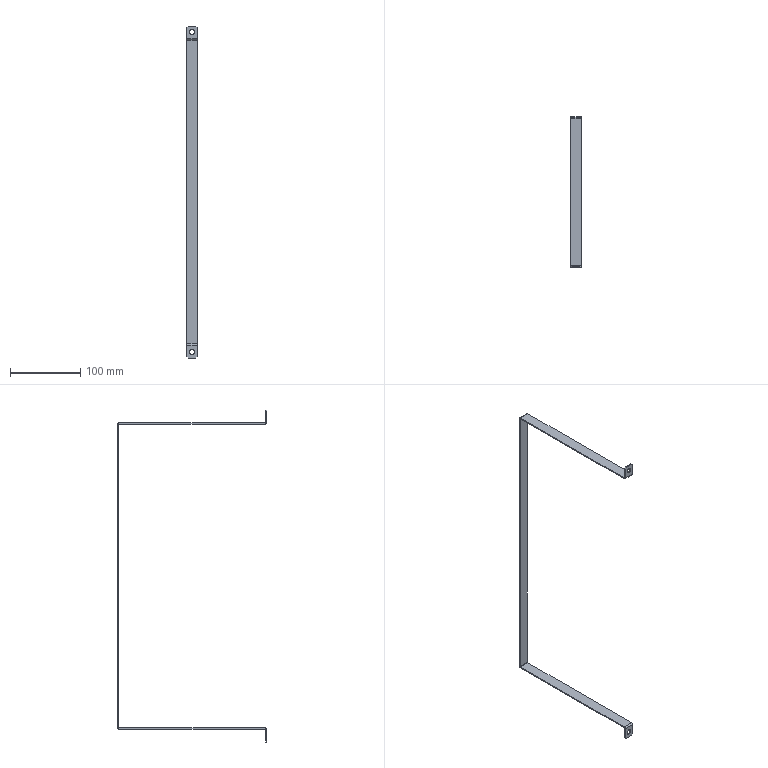Part | SolidWorks | features BaseBody 1 | 1 solid | 30 faces | box 15 x 213.5 x 473 mm | volume 19998 mm3 | plane 18 | cylinder 12 | commonest cylinder face diameters 1.473 x4 4.473 x4 7 x4
STEP:
#1=CARTESIAN_POINT('',(0.,1.5,-231.5));
#2=VERTEX_POINT('',#1);
#3=CARTESIAN_POINT('',(0.,1.5,-224.5));
#4=VERTEX_POINT('',#3);
#5=CARTESIAN_POINT('',(0.,1.5,-228.));
#6=DIRECTION('',(0.,1.,0.));
#7=DIRECTION('',(0.,0.,-1.));
#8=AXIS2_PLACEMENT_3D('',#5,#6,#7);
#9=CIRCLE('',#8,3.5);
#10=EDGE_CURVE('',#2,#4,#9,.T.);
#11=ORIENTED_EDGE('',*,*,#10,.T.);
#12=CARTESIAN_POINT('',(0.,0.,-224.5));
#13=VERTEX_POINT('',#12);
#14=CARTESIAN_POINT('',(0.,213.501,-224.5));
#15=DIRECTION('',(0.,-1.,0.));
#16=VECTOR('',#15,1000.);
#17=LINE('',#14,#16);
#18=EDGE_CURVE('',#4,#13,#17,.T.);
#19=ORIENTED_EDGE('',*,*,#18,.T.);
#20=CARTESIAN_POINT('',(0.,0.,-231.5));
#21=VERTEX_POINT('',#20);
#22=CARTESIAN_POINT('',(0.,0.,-228.));
#23=DIRECTION('',(0.,-1.,0.));
#24=DIRECTION('',(0.,0.,1.));
#25=AXIS2_PLACEMENT_3D('',#22,#23,#24);
#26=CIRCLE('',#25,3.5);
#27=EDGE_CURVE('',#13,#21,#26,.T.);
#28=ORIENTED_EDGE('',*,*,#27,.T.);
#29=CARTESIAN_POINT('',(0.,213.501,-231.5));
#30=DIRECTION('',(0.,-1.,0.));
#31=VECTOR('',#30,1000.);
#32=LINE('',#29,#31);
#33=EDGE_CURVE('',#2,#21,#32,.T.);
#34=ORIENTED_EDGE('',*,*,#33,.F.);
#35=EDGE_LOOP('',(#11,#19,#28,#34));
#36=FACE_OUTER_BOUND('',#35,.T.);
#37=CARTESIAN_POINT('',(0.,213.501,-228.));
#38=DIRECTION('',(0.,-1.,0.));
#39=DIRECTION('',(0.,0.,-1.));
#40=AXIS2_PLACEMENT_3D('',#37,#38,#39);
#41=CYLINDRICAL_SURFACE('',#40,3.5);
#42=ADVANCED_FACE('',(#36),#41,.F.);
#43=CARTESIAN_POINT('',(0.,1.5,224.5));
#44=VERTEX_POINT('',#43);
#45=CARTESIAN_POINT('',(0.,1.5,231.5));
#46=VERTEX_POINT('',#45);
#47=CARTESIAN_POINT('',(0.,1.5,228.));
#48=DIRECTION('',(0.,1.,0.));
#49=DIRECTION('',(0.,0.,-1.));
#50=AXIS2_PLACEMENT_3D('',#47,#48,#49);
#51=CIRCLE('',#50,3.5);
#52=EDGE_CURVE('',#44,#46,#51,.T.);
#53=ORIENTED_EDGE('',*,*,#52,.T.);
#54=CARTESIAN_POINT('',(0.,0.,231.5));
#55=VERTEX_POINT('',#54);
#56=CARTESIAN_POINT('',(0.,213.501,231.5));
#57=DIRECTION('',(0.,-1.,0.));
#58=VECTOR('',#57,1000.);
#59=LINE('',#56,#58);
#60=EDGE_CURVE('',#46,#55,#59,.T.);
#61=ORIENTED_EDGE('',*,*,#60,.T.);
#62=CARTESIAN_POINT('',(0.,0.,224.5));
#63=VERTEX_POINT('',#62);
#64=CARTESIAN_POINT('',(0.,0.,228.));
#65=DIRECTION('',(0.,-1.,0.));
#66=DIRECTION('',(0.,0.,-1.));
#67=AXIS2_PLACEMENT_3D('',#64,#65,#66);
#68=CIRCLE('',#67,3.5);
#69=EDGE_CURVE('',#55,#63,#68,.T.);
#70=ORIENTED_EDGE('',*,*,#69,.T.);
#71=CARTESIAN_POINT('',(0.,213.501,224.5));
#72=DIRECTION('',(0.,-1.,0.));
#73=VECTOR('',#72,1000.);
#74=LINE('',#71,#73);
#75=EDGE_CURVE('',#44,#63,#74,.T.);
#76=ORIENTED_EDGE('',*,*,#75,.F.);
#77=EDGE_LOOP('',(#53,#61,#70,#76));
#78=FACE_OUTER_BOUND('',#77,.T.);
#79=CARTESIAN_POINT('',(0.,213.501,228.));
#80=DIRECTION('',(0.,-1.,0.));
#81=DIRECTION('',(0.,0.,-1.));
#82=AXIS2_PLACEMENT_3D('',#79,#80,#81);
#83=CYLINDRICAL_SURFACE('',#82,3.5);
#84=ADVANCED_FACE('',(#78),#83,.F.);
#85=CARTESIAN_POINT('',(-5.5,0.,236.5));
#86=VERTEX_POINT('',#85);
#87=CARTESIAN_POINT('',(-7.5,0.,234.5));
#88=VERTEX_POINT('',#87);
#89=CARTESIAN_POINT('',(1.,0.,243.));
#90=DIRECTION('',(-0.7071,0.,-0.7071));
#91=VECTOR('',#90,1000.);
#92=LINE('',#89,#91);
#93=EDGE_CURVE('',#86,#88,#92,.T.);
#94=ORIENTED_EDGE('',*,*,#93,.F.);
#95=CARTESIAN_POINT('',(-5.5,1.5,236.5));
#96=VERTEX_POINT('',#95);
#97=CARTESIAN_POINT('',(-5.5,0.,236.5));
#98=DIRECTION('',(0.,-1.,0.));
#99=VECTOR('',#98,1000.);
#100=LINE('',#97,#99);
#101=EDGE_CURVE('',#96,#86,#100,.T.);
#102=ORIENTED_EDGE('',*,*,#101,.F.);
#103=CARTESIAN_POINT('',(-7.5,1.5,234.5));
#104=VERTEX_POINT('',#103);
#105=CARTESIAN_POINT('',(-7.5,1.5,234.5));
#106=DIRECTION('',(0.7071,0.,0.7071));
#107=VECTOR('',#106,1000.);
#108=LINE('',#105,#107);
#109=EDGE_CURVE('',#104,#96,#108,.T.);
#110=ORIENTED_EDGE('',*,*,#109,.F.);
#111=CARTESIAN_POINT('',(-7.5,2.237,234.5));
#112=DIRECTION('',(0.,1.,0.));
#113=VECTOR('',#112,1000.);
#114=LINE('',#111,#113);
#115=EDGE_CURVE('',#88,#104,#114,.T.);
#116=ORIENTED_EDGE('',*,*,#115,.F.);
#117=EDGE_LOOP('',(#94,#102,#110,#116));
#118=FACE_OUTER_BOUND('',#117,.T.);
#119=CARTESIAN_POINT('',(-7.5,2.237,234.5));
#120=DIRECTION('',(0.7071,0.,-0.7071));
#121=DIRECTION('',(0.,-1.,0.));
#122=AXIS2_PLACEMENT_3D('',#119,#120,#121);
#123=PLANE('',#122);
#124=ADVANCED_FACE('',(#118),#123,.F.);
#125=CARTESIAN_POINT('',(7.5,0.,234.5));
#126=VERTEX_POINT('',#125);
#127=CARTESIAN_POINT('',(5.5,0.,236.5));
#128=VERTEX_POINT('',#127);
#129=CARTESIAN_POINT('',(6.5,0.,235.5));
#130=DIRECTION('',(-0.7071,0.,0.7071));
#131=VECTOR('',#130,1000.);
#132=LINE('',#129,#131);
#133=EDGE_CURVE('',#126,#128,#132,.T.);
#134=ORIENTED_EDGE('',*,*,#133,.F.);
#135=CARTESIAN_POINT('',(7.5,1.5,234.5));
#136=VERTEX_POINT('',#135);
#137=CARTESIAN_POINT('',(7.5,2.237,234.5));
#138=DIRECTION('',(0.,-1.,0.));
#139=VECTOR('',#138,1000.);
#140=LINE('',#137,#139);
#141=EDGE_CURVE('',#136,#126,#140,.T.);
#142=ORIENTED_EDGE('',*,*,#141,.F.);
#143=CARTESIAN_POINT('',(5.5,1.5,236.5));
#144=VERTEX_POINT('',#143);
#145=CARTESIAN_POINT('',(5.5,1.5,236.5));
#146=DIRECTION('',(0.7071,0.,-0.7071));
#147=VECTOR('',#146,1000.);
#148=LINE('',#145,#147);
#149=EDGE_CURVE('',#144,#136,#148,.T.);
#150=ORIENTED_EDGE('',*,*,#149,.F.);
#151=CARTESIAN_POINT('',(5.5,0.,236.5));
#152=DIRECTION('',(0.,1.,0.));
#153=VECTOR('',#152,1000.);
#154=LINE('',#151,#153);
#155=EDGE_CURVE('',#128,#144,#154,.T.);
#156=ORIENTED_EDGE('',*,*,#155,.F.);
#157=EDGE_LOOP('',(#134,#142,#150,#156));
#158=FACE_OUTER_BOUND('',#157,.T.);
#159=CARTESIAN_POINT('',(5.5,0.,236.5));
#160=DIRECTION('',(-0.7071,0.,-0.7071));
#161=DIRECTION('',(-0.7071,0.,0.7071));
#162=AXIS2_PLACEMENT_3D('',#159,#160,#161);
#163=PLANE('',#162);
#164=ADVANCED_FACE('',(#158),#163,.F.);
#165=CARTESIAN_POINT('',(-5.5,1.5,-236.5));
#166=VERTEX_POINT('',#165);
#167=CARTESIAN_POINT('',(-7.5,1.5,-234.5));
#168=VERTEX_POINT('',#167);
#169=CARTESIAN_POINT('',(-7.5,1.5,-234.5));
#170=DIRECTION('',(-0.7071,0.,0.7071));
#171=VECTOR('',#170,1000.);
#172=LINE('',#169,#171);
#173=EDGE_CURVE('',#166,#168,#172,.T.);
#174=ORIENTED_EDGE('',*,*,#173,.F.);
#175=CARTESIAN_POINT('',(-5.5,0.,-236.5));
#176=VERTEX_POINT('',#175);
#177=CARTESIAN_POINT('',(-5.5,1.5,-236.5));
#178=DIRECTION('',(0.,1.,0.));
#179=VECTOR('',#178,1000.);
#180=LINE('',#177,#179);
#181=EDGE_CURVE('',#176,#166,#180,.T.);
#182=ORIENTED_EDGE('',*,*,#181,.F.);
#183=CARTESIAN_POINT('',(-7.5,0.,-234.5));
#184=VERTEX_POINT('',#183);
#185=CARTESIAN_POINT('',(1.,0.,-243.));
#186=DIRECTION('',(0.7071,0.,-0.7071));
#187=VECTOR('',#186,1000.);
#188=LINE('',#185,#187);
#189=EDGE_CURVE('',#184,#176,#188,.T.);
#190=ORIENTED_EDGE('',*,*,#189,.F.);
#191=CARTESIAN_POINT('',(-7.5,2.237,-234.5));
#192=DIRECTION('',(0.,-1.,0.));
#193=VECTOR('',#192,1000.);
#194=LINE('',#191,#193);
#195=EDGE_CURVE('',#168,#184,#194,.T.);
#196=ORIENTED_EDGE('',*,*,#195,.F.);
#197=EDGE_LOOP('',(#174,#182,#190,#196));
#198=FACE_OUTER_BOUND('',#197,.T.);
#199=CARTESIAN_POINT('',(-7.5,2.237,-234.5));
#200=DIRECTION('',(0.7071,0.,0.7071));
#201=DIRECTION('',(0.,-1.,0.));
#202=AXIS2_PLACEMENT_3D('',#199,#200,#201);
#203=PLANE('',#202);
#204=ADVANCED_FACE('',(#198),#203,.F.);
#205=CARTESIAN_POINT('',(7.5,1.5,-234.5));
#206=VERTEX_POINT('',#205);
#207=CARTESIAN_POINT('',(5.5,1.5,-236.5));
#208=VERTEX_POINT('',#207);
#209=CARTESIAN_POINT('',(5.5,1.5,-236.5));
#210=DIRECTION('',(-0.7071,0.,-0.7071));
#211=VECTOR('',#210,1000.);
#212=LINE('',#209,#211);
#213=EDGE_CURVE('',#206,#208,#212,.T.);
#214=ORIENTED_EDGE('',*,*,#213,.F.);
#215=CARTESIAN_POINT('',(7.5,0.,-234.5));
#216=VERTEX_POINT('',#215);
#217=CARTESIAN_POINT('',(7.5,1.5,-234.5));
#218=DIRECTION('',(0.,1.,0.));
#219=VECTOR('',#218,1000.);
#220=LINE('',#217,#219);
#221=EDGE_CURVE('',#216,#206,#220,.T.);
#222=ORIENTED_EDGE('',*,*,#221,.F.);
#223=CARTESIAN_POINT('',(5.5,0.,-236.5));
#224=VERTEX_POINT('',#223);
#225=CARTESIAN_POINT('',(6.5,0.,-235.5));
#226=DIRECTION('',(0.7071,0.,0.7071));
#227=VECTOR('',#226,1000.);
#228=LINE('',#225,#227);
#229=EDGE_CURVE('',#224,#216,#228,.T.);
#230=ORIENTED_EDGE('',*,*,#229,.F.);
#231=CARTESIAN_POINT('',(5.5,0.,-236.5));
#232=DIRECTION('',(0.,-1.,0.));
#233=VECTOR('',#232,1000.);
#234=LINE('',#231,#233);
#235=EDGE_CURVE('',#208,#224,#234,.T.);
#236=ORIENTED_EDGE('',*,*,#235,.F.);
#237=EDGE_LOOP('',(#214,#222,#230,#236));
#238=FACE_OUTER_BOUND('',#237,.T.);
#239=CARTESIAN_POINT('',(5.5,1.5,-236.5));
#240=DIRECTION('',(0.7071,0.,-0.7071));
#241=DIRECTION('',(0.,-1.,0.));
#242=AXIS2_PLACEMENT_3D('',#239,#240,#241);
#243=PLANE('',#242);
#244=ADVANCED_FACE('',(#238),#243,.T.);
#245=CARTESIAN_POINT('',(-7.5,2.237,218.));
#246=VERTEX_POINT('',#245);
#247=CARTESIAN_POINT('',(-7.5,1.5,218.737));
#248=VERTEX_POINT('',#247);
#249=CARTESIAN_POINT('',(-7.5,2.237,218.737));
#250=DIRECTION('',(-1.,0.,0.));
#251=DIRECTION('',(0.,0.,-1.));
#252=AXIS2_PLACEMENT_3D('',#249,#250,#251);
#253=CIRCLE('',#252,0.7366);
#254=EDGE_CURVE('',#246,#248,#253,.T.);
#255=ORIENTED_EDGE('',*,*,#254,.T.);
#256=CARTESIAN_POINT('',(7.5,1.5,218.737));
#257=VERTEX_POINT('',#256);
#258=CARTESIAN_POINT('',(7.5,1.5,218.737));
#259=DIRECTION('',(-1.,0.,0.));
#260=VECTOR('',#259,1000.);
#261=LINE('',#258,#260);
#262=EDGE_CURVE('',#257,#248,#261,.T.);
#263=ORIENTED_EDGE('',*,*,#262,.F.);
#264=CARTESIAN_POINT('',(7.5,2.237,218.));
#265=VERTEX_POINT('',#264);
#266=CARTESIAN_POINT('',(7.5,2.237,218.737));
#267=DIRECTION('',(-1.,0.,0.));
#268=DIRECTION('',(0.,0.,-1.));
#269=AXIS2_PLACEMENT_3D('',#266,#267,#268);
#270=CIRCLE('',#269,0.7366);
#271=EDGE_CURVE('',#265,#257,#270,.T.);
#272=ORIENTED_EDGE('',*,*,#271,.F.);
#273=CARTESIAN_POINT('',(7.5,2.237,218.));
#274=DIRECTION('',(-1.,0.,0.));
#275=VECTOR('',#274,1000.);
#276=LINE('',#273,#275);
#277=EDGE_CURVE('',#265,#246,#276,.T.);
#278=ORIENTED_EDGE('',*,*,#277,.T.);
#279=EDGE_LOOP('',(#255,#263,#272,#278));
#280=FACE_OUTER_BOUND('',#279,.T.);
#281=CARTESIAN_POINT('',(7.5,2.237,218.737));
#282=DIRECTION('',(-1.,0.,0.));
#283=DIRECTION('',(0.,0.,1.));
#284=AXIS2_PLACEMENT_3D('',#281,#282,#283);
#285=CYLINDRICAL_SURFACE('',#284,0.7366);
#286=ADVANCED_FACE('',(#280),#285,.F.);
#287=CARTESIAN_POINT('',(-7.5,211.263,218.));
#288=VERTEX_POINT('',#287);
#289=CARTESIAN_POINT('',(-7.5,0.,218.));
#290=DIRECTION('',(0.,-1.,0.));
#291=VECTOR('',#290,1000.);
#292=LINE('',#289,#291);
#293=EDGE_CURVE('',#288,#246,#292,.T.);
#294=ORIENTED_EDGE('',*,*,#293,.T.);
#295=ORIENTED_EDGE('',*,*,#277,.F.);
#296=CARTESIAN_POINT('',(7.5,211.263,218.));
#297=VERTEX_POINT('',#296);
#298=CARTESIAN_POINT('',(7.5,0.,218.));
#299=DIRECTION('',(0.,-1.,0.));
#300=VECTOR('',#299,1000.);
#301=LINE('',#298,#300);
#302=EDGE_CURVE('',#297,#265,#301,.T.);
#303=ORIENTED_EDGE('',*,*,#302,.F.);
#304=CARTESIAN_POINT('',(7.5,211.263,218.));
#305=DIRECTION('',(-1.,0.,0.));
#306=VECTOR('',#305,1000.);
#307=LINE('',#304,#306);
#308=EDGE_CURVE('',#297,#288,#307,.T.);
#309=ORIENTED_EDGE('',*,*,#308,.T.);
#310=EDGE_LOOP('',(#294,#295,#303,#309));
#311=FACE_OUTER_BOUND('',#310,.T.);
#312=CARTESIAN_POINT('',(7.5,0.,218.));
#313=DIRECTION('',(0.,0.,-1.));
#314=DIRECTION('',(0.,-1.,0.));
#315=AXIS2_PLACEMENT_3D('',#312,#313,#314);
#316=PLANE('',#315);
#317=ADVANCED_FACE('',(#311),#316,.F.);
#318=CARTESIAN_POINT('',(-7.5,213.5,215.763));
#319=VERTEX_POINT('',#318);
#320=CARTESIAN_POINT('',(-7.5,211.263,215.763));
#321=DIRECTION('',(1.,0.,0.));
#322=DIRECTION('',(0.,0.,-1.));
#323=AXIS2_PLACEMENT_3D('',#320,#321,#322);
#324=CIRCLE('',#323,2.237);
#325=EDGE_CURVE('',#319,#288,#324,.T.);
#326=ORIENTED_EDGE('',*,*,#325,.T.);
#327=ORIENTED_EDGE('',*,*,#308,.F.);
#328=CARTESIAN_POINT('',(7.5,213.5,215.763));
#329=VERTEX_POINT('',#328);
#330=CARTESIAN_POINT('',(7.5,211.263,215.763));
#331=DIRECTION('',(1.,0.,0.));
#332=DIRECTION('',(0.,0.,-1.));
#333=AXIS2_PLACEMENT_3D('',#330,#331,#332);
#334=CIRCLE('',#333,2.237);
#335=EDGE_CURVE('',#329,#297,#334,.T.);
#336=ORIENTED_EDGE('',*,*,#335,.F.);
#337=CARTESIAN_POINT('',(7.5,213.5,215.763));
#338=DIRECTION('',(-1.,0.,0.));
#339=VECTOR('',#338,1000.);
#340=LINE('',#337,#339);
#341=EDGE_CURVE('',#329,#319,#340,.T.);
#342=ORIENTED_EDGE('',*,*,#341,.T.);
#343=EDGE_LOOP('',(#326,#327,#336,#342));
#344=FACE_OUTER_BOUND('',#343,.T.);
#345=CARTESIAN_POINT('',(7.5,211.263,215.763));
#346=DIRECTION('',(-1.,0.,0.));
#347=DIRECTION('',(0.,0.,1.));
#348=AXIS2_PLACEMENT_3D('',#345,#346,#347);
#349=CYLINDRICAL_SURFACE('',#348,2.237);
#350=ADVANCED_FACE('',(#344),#349,.T.);
#351=CARTESIAN_POINT('',(-7.5,213.5,-215.763));
#352=VERTEX_POINT('',#351);
#353=CARTESIAN_POINT('',(-7.5,213.5,216.5));
#354=DIRECTION('',(0.,0.,1.));
#355=VECTOR('',#354,1000.);
#356=LINE('',#353,#355);
#357=EDGE_CURVE('',#352,#319,#356,.T.);
#358=ORIENTED_EDGE('',*,*,#357,.T.);
#359=ORIENTED_EDGE('',*,*,#341,.F.);
#360=CARTESIAN_POINT('',(7.5,213.5,-215.763));
#361=VERTEX_POINT('',#360);
#362=CARTESIAN_POINT('',(7.5,213.5,216.5));
#363=DIRECTION('',(0.,0.,1.));
#364=VECTOR('',#363,1000.);
#365=LINE('',#362,#364);
#366=EDGE_CURVE('',#361,#329,#365,.T.);
#367=ORIENTED_EDGE('',*,*,#366,.F.);
#368=CARTESIAN_POINT('',(7.5,213.5,-215.763));
#369=DIRECTION('',(-1.,0.,0.));
#370=VECTOR('',#369,1000.);
#371=LINE('',#368,#370);
#372=EDGE_CURVE('',#361,#352,#371,.T.);
#373=ORIENTED_EDGE('',*,*,#372,.T.);
#374=EDGE_LOOP('',(#358,#359,#367,#373));
#375=FACE_OUTER_BOUND('',#374,.T.);
#376=CARTESIAN_POINT('',(7.5,213.5,216.5));
#377=DIRECTION('',(0.,-1.,0.));
#378=DIRECTION('',(0.,0.,-1.));
#379=AXIS2_PLACEMENT_3D('',#376,#377,#378);
#380=PLANE('',#379);
#381=ADVANCED_FACE('',(#375),#380,.F.);
#382=CARTESIAN_POINT('',(-7.5,211.263,-218.));
#383=VERTEX_POINT('',#382);
#384=CARTESIAN_POINT('',(-7.5,211.263,-215.763));
#385=DIRECTION('',(1.,0.,0.));
#386=DIRECTION('',(0.,0.,-1.));
#387=AXIS2_PLACEMENT_3D('',#384,#385,#386);
#388=CIRCLE('',#387,2.237);
#389=EDGE_CURVE('',#383,#352,#388,.T.);
#390=ORIENTED_EDGE('',*,*,#389,.T.);
#391=ORIENTED_EDGE('',*,*,#372,.F.);
#392=CARTESIAN_POINT('',(7.5,211.263,-218.));
#393=VERTEX_POINT('',#392);
#394=CARTESIAN_POINT('',(7.5,211.263,-215.763));
#395=DIRECTION('',(1.,0.,0.));
#396=DIRECTION('',(0.,0.,-1.));
#397=AXIS2_PLACEMENT_3D('',#394,#395,#396);
#398=CIRCLE('',#397,2.237);
#399=EDGE_CURVE('',#393,#361,#398,.T.);
#400=ORIENTED_EDGE('',*,*,#399,.F.);
#401=CARTESIAN_POINT('',(7.5,211.263,-218.));
#402=DIRECTION('',(-1.,0.,0.));
#403=VECTOR('',#402,1000.);
#404=LINE('',#401,#403);
#405=EDGE_CURVE('',#393,#383,#404,.T.);
#406=ORIENTED_EDGE('',*,*,#405,.T.);
#407=EDGE_LOOP('',(#390,#391,#400,#406));
#408=FACE_OUTER_BOUND('',#407,.T.);
#409=CARTESIAN_POINT('',(7.5,211.263,-215.763));
#410=DIRECTION('',(-1.,0.,0.));
#411=DIRECTION('',(0.,0.,1.));
#412=AXIS2_PLACEMENT_3D('',#409,#410,#411);
#413=CYLINDRICAL_SURFACE('',#412,2.237);
#414=ADVANCED_FACE('',(#408),#413,.T.);
#415=CARTESIAN_POINT('',(-7.5,2.237,-218.));
#416=VERTEX_POINT('',#415);
#417=CARTESIAN_POINT('',(-7.5,0.,-218.));
#418=DIRECTION('',(0.,1.,0.));
#419=VECTOR('',#418,1000.);
#420=LINE('',#417,#419);
#421=EDGE_CURVE('',#416,#383,#420,.T.);
#422=ORIENTED_EDGE('',*,*,#421,.T.);
#423=ORIENTED_EDGE('',*,*,#405,.F.);
#424=CARTESIAN_POINT('',(7.5,2.237,-218.));
#425=VERTEX_POINT('',#424);
#426=CARTESIAN_POINT('',(7.5,0.,-218.));
#427=DIRECTION('',(0.,1.,0.));
#428=VECTOR('',#427,1000.);
#429=LINE('',#426,#428);
#430=EDGE_CURVE('',#425,#393,#429,.T.);
#431=ORIENTED_EDGE('',*,*,#430,.F.);
#432=CARTESIAN_POINT('',(7.5,2.237,-218.));
#433=DIRECTION('',(-1.,0.,0.));
#434=VECTOR('',#433,1000.);
#435=LINE('',#432,#434);
#436=EDGE_CURVE('',#425,#416,#435,.T.);
#437=ORIENTED_EDGE('',*,*,#436,.T.);
#438=EDGE_LOOP('',(#422,#423,#431,#437));
#439=FACE_OUTER_BOUND('',#438,.T.);
#440=CARTESIAN_POINT('',(7.5,0.,-218.));
#441=DIRECTION('',(0.,0.,1.));
#442=DIRECTION('',(0.,-1.,0.));
#443=AXIS2_PLACEMENT_3D('',#440,#441,#442);
#444=PLANE('',#443);
#445=ADVANCED_FACE('',(#439),#444,.F.);
#446=CARTESIAN_POINT('',(-7.5,1.5,-218.737));
#447=VERTEX_POINT('',#446);
#448=CARTESIAN_POINT('',(-7.5,2.237,-218.737));
#449=DIRECTION('',(-1.,0.,0.));
#450=DIRECTION('',(0.,0.,-1.));
#451=AXIS2_PLACEMENT_3D('',#448,#449,#450);
#452=CIRCLE('',#451,0.7366);
#453=EDGE_CURVE('',#447,#416,#452,.T.);
#454=ORIENTED_EDGE('',*,*,#453,.T.);
#455=ORIENTED_EDGE('',*,*,#436,.F.);
#456=CARTESIAN_POINT('',(7.5,1.5,-218.737));
#457=VERTEX_POINT('',#456);
#458=CARTESIAN_POINT('',(7.5,2.237,-218.737));
#459=DIRECTION('',(-1.,0.,0.));
#460=DIRECTION('',(0.,0.,-1.));
#461=AXIS2_PLACEMENT_3D('',#458,#459,#460);
#462=CIRCLE('',#461,0.7366);
#463=EDGE_CURVE('',#457,#425,#462,.T.);
#464=ORIENTED_EDGE('',*,*,#463,.F.);
#465=CARTESIAN_POINT('',(7.5,1.5,-218.737));
#466=DIRECTION('',(-1.,0.,0.));
#467=VECTOR('',#466,1000.);
#468=LINE('',#465,#467);
#469=EDGE_CURVE('',#457,#447,#468,.T.);
#470=ORIENTED_EDGE('',*,*,#469,.T.);
#471=EDGE_LOOP('',(#454,#455,#464,#470));
#472=FACE_OUTER_BOUND('',#471,.T.);
#473=CARTESIAN_POINT('',(7.5,2.237,-218.737));
#474=DIRECTION('',(-1.,0.,0.));
#475=DIRECTION('',(0.,0.,1.));
#476=AXIS2_PLACEMENT_3D('',#473,#474,#475);
#477=CYLINDRICAL_SURFACE('',#476,0.7366);
#478=ADVANCED_FACE('',(#472),#477,.F.);
#479=ORIENTED_EDGE('',*,*,#10,.F.);
#480=CARTESIAN_POINT('',(0.,1.5,-228.));
#481=DIRECTION('',(0.,1.,0.));
#482=DIRECTION('',(0.,0.,-1.));
#483=AXIS2_PLACEMENT_3D('',#480,#481,#482);
#484=CIRCLE('',#483,3.5);
#485=EDGE_CURVE('',#4,#2,#484,.T.);
#486=ORIENTED_EDGE('',*,*,#485,.F.);
#487=EDGE_LOOP('',(#479,#486));
#488=FACE_BOUND('',#487,.T.);
#489=CARTESIAN_POINT('',(7.5,1.5,-236.5));
#490=DIRECTION('',(0.,0.,1.));
#491=VECTOR('',#490,1000.);
#492=LINE('',#489,#491);
#493=EDGE_CURVE('',#206,#457,#492,.T.);
#494=ORIENTED_EDGE('',*,*,#493,.F.);
#495=ORIENTED_EDGE('',*,*,#213,.T.);
#496=CARTESIAN_POINT('',(7.5,1.5,-236.5));
#497=DIRECTION('',(-1.,0.,0.));
#498=VECTOR('',#497,1000.);
#499=LINE('',#496,#498);
#500=EDGE_CURVE('',#208,#166,#499,.T.);
#501=ORIENTED_EDGE('',*,*,#500,.T.);
#502=ORIENTED_EDGE('',*,*,#173,.T.);
#503=CARTESIAN_POINT('',(-7.5,1.5,-236.5));
#504=DIRECTION('',(0.,0.,1.));
#505=VECTOR('',#504,1000.);
#506=LINE('',#503,#505);
#507=EDGE_CURVE('',#168,#447,#506,.T.);
#508=ORIENTED_EDGE('',*,*,#507,.T.);
#509=ORIENTED_EDGE('',*,*,#469,.F.);
#510=EDGE_LOOP('',(#494,#495,#501,#502,#508,#509));
#511=FACE_OUTER_BOUND('',#510,.T.);
#512=CARTESIAN_POINT('',(7.5,1.5,-236.5));
#513=DIRECTION('',(0.,-1.,0.));
#514=DIRECTION('',(0.,0.,-1.));
#515=AXIS2_PLACEMENT_3D('',#512,#513,#514);
#516=PLANE('',#515);
#517=ADVANCED_FACE('',(#488,#511),#516,.F.);
#518=ORIENTED_EDGE('',*,*,#500,.F.);
#519=ORIENTED_EDGE('',*,*,#235,.T.);
#520=CARTESIAN_POINT('',(7.5,0.,-236.5));
#521=DIRECTION('',(-1.,0.,0.));
#522=VECTOR('',#521,1000.);
#523=LINE('',#520,#522);
#524=EDGE_CURVE('',#224,#176,#523,.T.);
#525=ORIENTED_EDGE('',*,*,#524,.T.);
#526=ORIENTED_EDGE('',*,*,#181,.T.);
#527=EDGE_LOOP('',(#518,#519,#525,#526));
#528=FACE_OUTER_BOUND('',#527,.T.);
#529=CARTESIAN_POINT('',(7.5,1.5,-236.5));
#530=DIRECTION('',(0.,0.,-1.));
#531=DIRECTION('',(0.,-1.,0.));
#532=AXIS2_PLACEMENT_3D('',#529,#530,#531);
#533=PLANE('',#532);
#534=ADVANCED_FACE('',(#528),#533,.T.);
#535=CARTESIAN_POINT('',(0.,0.,-228.));
#536=DIRECTION('',(0.,-1.,0.));
#537=DIRECTION('',(0.,0.,1.));
#538=AXIS2_PLACEMENT_3D('',#535,#536,#537);
#539=CIRCLE('',#538,3.5);
#540=EDGE_CURVE('',#21,#13,#539,.T.);
#541=ORIENTED_EDGE('',*,*,#540,.F.);
#542=ORIENTED_EDGE('',*,*,#27,.F.);
#543=EDGE_LOOP('',(#541,#542));
#544=FACE_BOUND('',#543,.T.);
#545=ORIENTED_EDGE('',*,*,#524,.F.);
#546=ORIENTED_EDGE('',*,*,#229,.T.);
#547=CARTESIAN_POINT('',(7.5,0.,-218.737));
#548=VERTEX_POINT('',#547);
#549=CARTESIAN_POINT('',(7.5,0.,-236.5));
#550=DIRECTION('',(0.,0.,1.));
#551=VECTOR('',#550,1000.);
#552=LINE('',#549,#551);
#553=EDGE_CURVE('',#216,#548,#552,.T.);
#554=ORIENTED_EDGE('',*,*,#553,.T.);
#555=CARTESIAN_POINT('',(-7.5,0.,-218.737));
#556=VERTEX_POINT('',#555);
#557=CARTESIAN_POINT('',(7.5,0.,-218.737));
#558=DIRECTION('',(-1.,0.,0.));
#559=VECTOR('',#558,1000.);
#560=LINE('',#557,#559);
#561=EDGE_CURVE('',#548,#556,#560,.T.);
#562=ORIENTED_EDGE('',*,*,#561,.T.);
#563=CARTESIAN_POINT('',(-7.5,0.,-236.5));
#564=DIRECTION('',(0.,0.,1.));
#565=VECTOR('',#564,1000.);
#566=LINE('',#563,#565);
#567=EDGE_CURVE('',#184,#556,#566,.T.);
#568=ORIENTED_EDGE('',*,*,#567,.F.);
#569=ORIENTED_EDGE('',*,*,#189,.T.);
#570=EDGE_LOOP('',(#545,#546,#554,#562,#568,#569));
#571=FACE_OUTER_BOUND('',#570,.T.);
#572=CARTESIAN_POINT('',(7.5,0.,-236.5));
#573=DIRECTION('',(0.,-1.,0.));
#574=DIRECTION('',(0.,0.,-1.));
#575=AXIS2_PLACEMENT_3D('',#572,#573,#574);
#576=PLANE('',#575);
#577=ADVANCED_FACE('',(#544,#571),#576,.T.);
#578=CARTESIAN_POINT('',(-7.5,2.237,-216.5));
#579=VERTEX_POINT('',#578);
#580=CARTESIAN_POINT('',(-7.5,2.237,-218.737));
#581=DIRECTION('',(-1.,0.,0.));
#582=DIRECTION('',(0.,0.,1.));
#583=AXIS2_PLACEMENT_3D('',#580,#581,#582);
#584=CIRCLE('',#583,2.237);
#585=EDGE_CURVE('',#556,#579,#584,.T.);
#586=ORIENTED_EDGE('',*,*,#585,.F.);
#587=ORIENTED_EDGE('',*,*,#561,.F.);
#588=CARTESIAN_POINT('',(7.5,2.237,-216.5));
#589=VERTEX_POINT('',#588);
#590=CARTESIAN_POINT('',(7.5,2.237,-218.737));
#591=DIRECTION('',(-1.,0.,0.));
#592=DIRECTION('',(0.,0.,1.));
#593=AXIS2_PLACEMENT_3D('',#590,#591,#592);
#594=CIRCLE('',#593,2.237);
#595=EDGE_CURVE('',#548,#589,#594,.T.);
#596=ORIENTED_EDGE('',*,*,#595,.T.);
#597=CARTESIAN_POINT('',(7.5,2.237,-216.5));
#598=DIRECTION('',(-1.,0.,0.));
#599=VECTOR('',#598,1000.);
#600=LINE('',#597,#599);
#601=EDGE_CURVE('',#589,#579,#600,.T.);
#602=ORIENTED_EDGE('',*,*,#601,.T.);
#603=EDGE_LOOP('',(#586,#587,#596,#602));
#604=FACE_OUTER_BOUND('',#603,.T.);
#605=CARTESIAN_POINT('',(7.5,2.237,-218.737));
#606=DIRECTION('',(-1.,0.,0.));
#607=DIRECTION('',(0.,0.,1.));
#608=AXIS2_PLACEMENT_3D('',#605,#606,#607);
#609=CYLINDRICAL_SURFACE('',#608,2.237);
#610=ADVANCED_FACE('',(#604),#609,.T.);
#611=CARTESIAN_POINT('',(-7.5,211.263,-216.5));
#612=VERTEX_POINT('',#611);
#613=CARTESIAN_POINT('',(-7.5,0.,-216.5));
#614=DIRECTION('',(0.,1.,0.));
#615=VECTOR('',#614,1000.);
#616=LINE('',#613,#615);
#617=EDGE_CURVE('',#579,#612,#616,.T.);
#618=ORIENTED_EDGE('',*,*,#617,.F.);
#619=ORIENTED_EDGE('',*,*,#601,.F.);
#620=CARTESIAN_POINT('',(7.5,211.263,-216.5));
#621=VERTEX_POINT('',#620);
#622=CARTESIAN_POINT('',(7.5,0.,-216.5));
#623=DIRECTION('',(0.,1.,0.));
#624=VECTOR('',#623,1000.);
#625=LINE('',#622,#624);
#626=EDGE_CURVE('',#589,#621,#625,.T.);
#627=ORIENTED_EDGE('',*,*,#626,.T.);
#628=CARTESIAN_POINT('',(7.5,211.263,-216.5));
#629=DIRECTION('',(-1.,0.,0.));
#630=VECTOR('',#629,1000.);
#631=LINE('',#628,#630);
#632=EDGE_CURVE('',#621,#612,#631,.T.);
#633=ORIENTED_EDGE('',*,*,#632,.T.);
#634=EDGE_LOOP('',(#618,#619,#627,#633));
#635=FACE_OUTER_BOUND('',#634,.T.);
#636=CARTESIAN_POINT('',(7.5,0.,-216.5));
#637=DIRECTION('',(0.,0.,1.));
#638=DIRECTION('',(0.,-1.,0.));
#639=AXIS2_PLACEMENT_3D('',#636,#637,#638);
#640=PLANE('',#639);
#641=ADVANCED_FACE('',(#635),#640,.T.);
#642=CARTESIAN_POINT('',(-7.5,212.,-215.763));
#643=VERTEX_POINT('',#642);
#644=CARTESIAN_POINT('',(-7.5,211.263,-215.763));
#645=DIRECTION('',(1.,0.,0.));
#646=DIRECTION('',(0.,0.,-1.));
#647=AXIS2_PLACEMENT_3D('',#644,#645,#646);
#648=CIRCLE('',#647,0.7366);
#649=EDGE_CURVE('',#612,#643,#648,.T.);
#650=ORIENTED_EDGE('',*,*,#649,.F.);
#651=ORIENTED_EDGE('',*,*,#632,.F.);
#652=CARTESIAN_POINT('',(7.5,212.,-215.763));
#653=VERTEX_POINT('',#652);
#654=CARTESIAN_POINT('',(7.5,211.263,-215.763));
#655=DIRECTION('',(1.,0.,0.));
#656=DIRECTION('',(0.,0.,-1.));
#657=AXIS2_PLACEMENT_3D('',#654,#655,#656);
#658=CIRCLE('',#657,0.7366);
#659=EDGE_CURVE('',#621,#653,#658,.T.);
#660=ORIENTED_EDGE('',*,*,#659,.T.);
#661=CARTESIAN_POINT('',(7.5,212.,-215.763));
#662=DIRECTION('',(-1.,0.,0.));
#663=VECTOR('',#662,1000.);
#664=LINE('',#661,#663);
#665=EDGE_CURVE('',#653,#643,#664,.T.);
#666=ORIENTED_EDGE('',*,*,#665,.T.);
#667=EDGE_LOOP('',(#650,#651,#660,#666));
#668=FACE_OUTER_BOUND('',#667,.T.);
#669=CARTESIAN_POINT('',(7.5,211.263,-215.763));
#670=DIRECTION('',(-1.,0.,0.));
#671=DIRECTION('',(0.,0.,1.));
#672=AXIS2_PLACEMENT_3D('',#669,#670,#671);
#673=CYLINDRICAL_SURFACE('',#672,0.7366);
#674=ADVANCED_FACE('',(#668),#673,.F.);
#675=CARTESIAN_POINT('',(-7.5,212.,215.763));
#676=VERTEX_POINT('',#675);
#677=CARTESIAN_POINT('',(-7.5,212.,216.5));
#678=DIRECTION('',(0.,0.,1.));
#679=VECTOR('',#678,1000.);
#680=LINE('',#677,#679);
#681=EDGE_CURVE('',#643,#676,#680,.T.);
#682=ORIENTED_EDGE('',*,*,#681,.F.);
#683=ORIENTED_EDGE('',*,*,#665,.F.);
#684=CARTESIAN_POINT('',(7.5,212.,215.763));
#685=VERTEX_POINT('',#684);
#686=CARTESIAN_POINT('',(7.5,212.,216.5));
#687=DIRECTION('',(0.,0.,1.));
#688=VECTOR('',#687,1000.);
#689=LINE('',#686,#688);
#690=EDGE_CURVE('',#653,#685,#689,.T.);
#691=ORIENTED_EDGE('',*,*,#690,.T.);
#692=CARTESIAN_POINT('',(7.5,212.,215.763));
#693=DIRECTION('',(-1.,0.,0.));
#694=VECTOR('',#693,1000.);
#695=LINE('',#692,#694);
#696=EDGE_CURVE('',#685,#676,#695,.T.);
#697=ORIENTED_EDGE('',*,*,#696,.T.);
#698=EDGE_LOOP('',(#682,#683,#691,#697));
#699=FACE_OUTER_BOUND('',#698,.T.);
#700=CARTESIAN_POINT('',(7.5,212.,216.5));
#701=DIRECTION('',(0.,-1.,0.));
#702=DIRECTION('',(0.,0.,-1.));
#703=AXIS2_PLACEMENT_3D('',#700,#701,#702);
#704=PLANE('',#703);
#705=ADVANCED_FACE('',(#699),#704,.T.);
#706=CARTESIAN_POINT('',(-7.5,211.263,216.5));
#707=VERTEX_POINT('',#706);
#708=CARTESIAN_POINT('',(-7.5,211.263,215.763));
#709=DIRECTION('',(1.,0.,0.));
#710=DIRECTION('',(0.,0.,-1.));
#711=AXIS2_PLACEMENT_3D('',#708,#709,#710);
#712=CIRCLE('',#711,0.7366);
#713=EDGE_CURVE('',#676,#707,#712,.T.);
#714=ORIENTED_EDGE('',*,*,#713,.F.);
#715=ORIENTED_EDGE('',*,*,#696,.F.);
#716=CARTESIAN_POINT('',(7.5,211.263,216.5));
#717=VERTEX_POINT('',#716);
#718=CARTESIAN_POINT('',(7.5,211.263,215.763));
#719=DIRECTION('',(1.,0.,0.));
#720=DIRECTION('',(0.,0.,-1.));
#721=AXIS2_PLACEMENT_3D('',#718,#719,#720);
#722=CIRCLE('',#721,0.7366);
#723=EDGE_CURVE('',#685,#717,#722,.T.);
#724=ORIENTED_EDGE('',*,*,#723,.T.);
#725=CARTESIAN_POINT('',(7.5,211.263,216.5));
#726=DIRECTION('',(-1.,0.,0.));
#727=VECTOR('',#726,1000.);
#728=LINE('',#725,#727);
#729=EDGE_CURVE('',#717,#707,#728,.T.);
#730=ORIENTED_EDGE('',*,*,#729,.T.);
#731=EDGE_LOOP('',(#714,#715,#724,#730));
#732=FACE_OUTER_BOUND('',#731,.T.);
#733=CARTESIAN_POINT('',(7.5,211.263,215.763));
#734=DIRECTION('',(-1.,0.,0.));
#735=DIRECTION('',(0.,0.,1.));
#736=AXIS2_PLACEMENT_3D('',#733,#734,#735);
#737=CYLINDRICAL_SURFACE('',#736,0.7366);
#738=ADVANCED_FACE('',(#732),#737,.F.);
#739=CARTESIAN_POINT('',(-7.5,2.237,216.5));
#740=VERTEX_POINT('',#739);
#741=CARTESIAN_POINT('',(-7.5,0.,216.5));
#742=DIRECTION('',(0.,-1.,0.));
#743=VECTOR('',#742,1000.);
#744=LINE('',#741,#743);
#745=EDGE_CURVE('',#707,#740,#744,.T.);
#746=ORIENTED_EDGE('',*,*,#745,.F.);
#747=ORIENTED_EDGE('',*,*,#729,.F.);
#748=CARTESIAN_POINT('',(7.5,2.237,216.5));
#749=VERTEX_POINT('',#748);
#750=CARTESIAN_POINT('',(7.5,0.,216.5));
#751=DIRECTION('',(0.,-1.,0.));
#752=VECTOR('',#751,1000.);
#753=LINE('',#750,#752);
#754=EDGE_CURVE('',#717,#749,#753,.T.);
#755=ORIENTED_EDGE('',*,*,#754,.T.);
#756=CARTESIAN_POINT('',(7.5,2.237,216.5));
#757=DIRECTION('',(-1.,0.,0.));
#758=VECTOR('',#757,1000.);
#759=LINE('',#756,#758);
#760=EDGE_CURVE('',#749,#740,#759,.T.);
#761=ORIENTED_EDGE('',*,*,#760,.T.);
#762=EDGE_LOOP('',(#746,#747,#755,#761));
#763=FACE_OUTER_BOUND('',#762,.T.);
#764=CARTESIAN_POINT('',(7.5,0.,216.5));
#765=DIRECTION('',(0.,0.,-1.));
#766=DIRECTION('',(0.,-1.,0.));
#767=AXIS2_PLACEMENT_3D('',#764,#765,#766);
#768=PLANE('',#767);
#769=ADVANCED_FACE('',(#763),#768,.T.);
#770=CARTESIAN_POINT('',(-7.5,0.,218.737));
#771=VERTEX_POINT('',#770);
#772=CARTESIAN_POINT('',(-7.5,2.237,218.737));
#773=DIRECTION('',(-1.,0.,0.));
#774=DIRECTION('',(0.,0.,1.));
#775=AXIS2_PLACEMENT_3D('',#772,#773,#774);
#776=CIRCLE('',#775,2.237);
#777=EDGE_CURVE('',#740,#771,#776,.T.);
#778=ORIENTED_EDGE('',*,*,#777,.F.);
#779=ORIENTED_EDGE('',*,*,#760,.F.);
#780=CARTESIAN_POINT('',(7.5,0.,218.737));
#781=VERTEX_POINT('',#780);
#782=CARTESIAN_POINT('',(7.5,2.237,218.737));
#783=DIRECTION('',(-1.,0.,0.));
#784=DIRECTION('',(0.,0.,1.));
#785=AXIS2_PLACEMENT_3D('',#782,#783,#784);
#786=CIRCLE('',#785,2.237);
#787=EDGE_CURVE('',#749,#781,#786,.T.);
#788=ORIENTED_EDGE('',*,*,#787,.T.);
#789=CARTESIAN_POINT('',(7.5,0.,218.737));
#790=DIRECTION('',(-1.,0.,0.));
#791=VECTOR('',#790,1000.);
#792=LINE('',#789,#791);
#793=EDGE_CURVE('',#781,#771,#792,.T.);
#794=ORIENTED_EDGE('',*,*,#793,.T.);
#795=EDGE_LOOP('',(#778,#779,#788,#794));
#796=FACE_OUTER_BOUND('',#795,.T.);
#797=CARTESIAN_POINT('',(7.5,2.237,218.737));
#798=DIRECTION('',(-1.,0.,0.));
#799=DIRECTION('',(0.,0.,1.));
#800=AXIS2_PLACEMENT_3D('',#797,#798,#799);
#801=CYLINDRICAL_SURFACE('',#800,2.237);
#802=ADVANCED_FACE('',(#796),#801,.T.);
#803=CARTESIAN_POINT('',(0.,0.,228.));
#804=DIRECTION('',(0.,-1.,0.));
#805=DIRECTION('',(0.,0.,-1.));
#806=AXIS2_PLACEMENT_3D('',#803,#804,#805);
#807=CIRCLE('',#806,3.5);
#808=EDGE_CURVE('',#63,#55,#807,.T.);
#809=ORIENTED_EDGE('',*,*,#808,.F.);
#810=ORIENTED_EDGE('',*,*,#69,.F.);
#811=EDGE_LOOP('',(#809,#810));
#812=FACE_BOUND('',#811,.T.);
#813=CARTESIAN_POINT('',(7.5,0.,236.5));
#814=DIRECTION('',(0.,0.,1.));
#815=VECTOR('',#814,1000.);
#816=LINE('',#813,#815);
#817=EDGE_CURVE('',#781,#126,#816,.T.);
#818=ORIENTED_EDGE('',*,*,#817,.T.);
#819=ORIENTED_EDGE('',*,*,#133,.T.);
#820=CARTESIAN_POINT('',(7.5,0.,236.5));
#821=DIRECTION('',(-1.,0.,0.));
#822=VECTOR('',#821,1000.);
#823=LINE('',#820,#822);
#824=EDGE_CURVE('',#128,#86,#823,.T.);
#825=ORIENTED_EDGE('',*,*,#824,.T.);
#826=ORIENTED_EDGE('',*,*,#93,.T.);
#827=CARTESIAN_POINT('',(-7.5,0.,236.5));
#828=DIRECTION('',(0.,0.,1.));
#829=VECTOR('',#828,1000.);
#830=LINE('',#827,#829);
#831=EDGE_CURVE('',#771,#88,#830,.T.);
#832=ORIENTED_EDGE('',*,*,#831,.F.);
#833=ORIENTED_EDGE('',*,*,#793,.F.);
#834=EDGE_LOOP('',(#818,#819,#825,#826,#832,#833));
#835=FACE_OUTER_BOUND('',#834,.T.);
#836=CARTESIAN_POINT('',(7.5,0.,236.5));
#837=DIRECTION('',(0.,-1.,0.));
#838=DIRECTION('',(-1.,0.,0.));
#839=AXIS2_PLACEMENT_3D('',#836,#837,#838);
#840=PLANE('',#839);
#841=ADVANCED_FACE('',(#812,#835),#840,.T.);
#842=ORIENTED_EDGE('',*,*,#824,.F.);
#843=ORIENTED_EDGE('',*,*,#155,.T.);
#844=CARTESIAN_POINT('',(7.5,1.5,236.5));
#845=DIRECTION('',(-1.,0.,0.));
#846=VECTOR('',#845,1000.);
#847=LINE('',#844,#846);
#848=EDGE_CURVE('',#144,#96,#847,.T.);
#849=ORIENTED_EDGE('',*,*,#848,.T.);
#850=ORIENTED_EDGE('',*,*,#101,.T.);
#851=EDGE_LOOP('',(#842,#843,#849,#850));
#852=FACE_OUTER_BOUND('',#851,.T.);
#853=CARTESIAN_POINT('',(7.5,0.,236.5));
#854=DIRECTION('',(0.,0.,1.));
#855=DIRECTION('',(1.,0.,0.));
#856=AXIS2_PLACEMENT_3D('',#853,#854,#855);
#857=PLANE('',#856);
#858=ADVANCED_FACE('',(#852),#857,.T.);
#859=ORIENTED_EDGE('',*,*,#52,.F.);
#860=CARTESIAN_POINT('',(0.,1.5,228.));
#861=DIRECTION('',(0.,1.,0.));
#862=DIRECTION('',(0.,0.,-1.));
#863=AXIS2_PLACEMENT_3D('',#860,#861,#862);
#864=CIRCLE('',#863,3.5);
#865=EDGE_CURVE('',#46,#44,#864,.T.);
#866=ORIENTED_EDGE('',*,*,#865,.F.);
#867=EDGE_LOOP('',(#859,#866));
#868=FACE_BOUND('',#867,.T.);
#869=ORIENTED_EDGE('',*,*,#848,.F.);
#870=ORIENTED_EDGE('',*,*,#149,.T.);
#871=CARTESIAN_POINT('',(7.5,1.5,236.5));
#872=DIRECTION('',(0.,0.,1.));
#873=VECTOR('',#872,1000.);
#874=LINE('',#871,#873);
#875=EDGE_CURVE('',#257,#136,#874,.T.);
#876=ORIENTED_EDGE('',*,*,#875,.F.);
#877=ORIENTED_EDGE('',*,*,#262,.T.);
#878=CARTESIAN_POINT('',(-7.5,1.5,236.5));
#879=DIRECTION('',(0.,0.,1.));
#880=VECTOR('',#879,1000.);
#881=LINE('',#878,#880);
#882=EDGE_CURVE('',#248,#104,#881,.T.);
#883=ORIENTED_EDGE('',*,*,#882,.T.);
#884=ORIENTED_EDGE('',*,*,#109,.T.);
#885=EDGE_LOOP('',(#869,#870,#876,#877,#883,#884));
#886=FACE_OUTER_BOUND('',#885,.T.);
#887=CARTESIAN_POINT('',(7.5,1.5,236.5));
#888=DIRECTION('',(0.,-1.,0.));
#889=DIRECTION('',(-1.,0.,0.));
#890=AXIS2_PLACEMENT_3D('',#887,#888,#889);
#891=PLANE('',#890);
#892=ADVANCED_FACE('',(#868,#886),#891,.F.);
#893=ORIENTED_EDGE('',*,*,#254,.F.);
#894=ORIENTED_EDGE('',*,*,#293,.F.);
#895=ORIENTED_EDGE('',*,*,#325,.F.);
#896=ORIENTED_EDGE('',*,*,#357,.F.);
#897=ORIENTED_EDGE('',*,*,#389,.F.);
#898=ORIENTED_EDGE('',*,*,#421,.F.);
#899=ORIENTED_EDGE('',*,*,#453,.F.);
#900=ORIENTED_EDGE('',*,*,#507,.F.);
#901=ORIENTED_EDGE('',*,*,#195,.T.);
#902=ORIENTED_EDGE('',*,*,#567,.T.);
#903=ORIENTED_EDGE('',*,*,#585,.T.);
#904=ORIENTED_EDGE('',*,*,#617,.T.);
#905=ORIENTED_EDGE('',*,*,#649,.T.);
#906=ORIENTED_EDGE('',*,*,#681,.T.);
#907=ORIENTED_EDGE('',*,*,#713,.T.);
#908=ORIENTED_EDGE('',*,*,#745,.T.);
#909=ORIENTED_EDGE('',*,*,#777,.T.);
#910=ORIENTED_EDGE('',*,*,#831,.T.);
#911=ORIENTED_EDGE('',*,*,#115,.T.);
#912=ORIENTED_EDGE('',*,*,#882,.F.);
#913=EDGE_LOOP('',(#893,#894,#895,#896,#897,#898,#899,#900,#901,#902,#903,#904,#905,#906,#907,#908,#909,#910,#911,#912));
#914=FACE_OUTER_BOUND('',#913,.T.);
#915=CARTESIAN_POINT('',(-7.5,2.237,216.5));
#916=DIRECTION('',(-1.,0.,0.));
#917=DIRECTION('',(0.,0.,1.));
#918=AXIS2_PLACEMENT_3D('',#915,#916,#917);
#919=PLANE('',#918);
#920=ADVANCED_FACE('',(#914),#919,.T.);
#921=ORIENTED_EDGE('',*,*,#271,.T.);
#922=ORIENTED_EDGE('',*,*,#875,.T.);
#923=ORIENTED_EDGE('',*,*,#141,.T.);
#924=ORIENTED_EDGE('',*,*,#817,.F.);
#925=ORIENTED_EDGE('',*,*,#787,.F.);
#926=ORIENTED_EDGE('',*,*,#754,.F.);
#927=ORIENTED_EDGE('',*,*,#723,.F.);
#928=ORIENTED_EDGE('',*,*,#690,.F.);
#929=ORIENTED_EDGE('',*,*,#659,.F.);
#930=ORIENTED_EDGE('',*,*,#626,.F.);
#931=ORIENTED_EDGE('',*,*,#595,.F.);
#932=ORIENTED_EDGE('',*,*,#553,.F.);
#933=ORIENTED_EDGE('',*,*,#221,.T.);
#934=ORIENTED_EDGE('',*,*,#493,.T.);
#935=ORIENTED_EDGE('',*,*,#463,.T.);
#936=ORIENTED_EDGE('',*,*,#430,.T.);
#937=ORIENTED_EDGE('',*,*,#399,.T.);
#938=ORIENTED_EDGE('',*,*,#366,.T.);
#939=ORIENTED_EDGE('',*,*,#335,.T.);
#940=ORIENTED_EDGE('',*,*,#302,.T.);
#941=EDGE_LOOP('',(#921,#922,#923,#924,#925,#926,#927,#928,#929,#930,#931,#932,#933,#934,#935,#936,#937,#938,#939,#940));
#942=FACE_OUTER_BOUND('',#941,.T.);
#943=CARTESIAN_POINT('',(7.5,0.,218.737));
#944=DIRECTION('',(1.,0.,0.));
#945=DIRECTION('',(0.,1.,0.));
#946=AXIS2_PLACEMENT_3D('',#943,#944,#945);
#947=PLANE('',#946);
#948=ADVANCED_FACE('',(#942),#947,.T.);
#949=ORIENTED_EDGE('',*,*,#60,.F.);
#950=ORIENTED_EDGE('',*,*,#865,.T.);
#951=ORIENTED_EDGE('',*,*,#75,.T.);
#952=ORIENTED_EDGE('',*,*,#808,.T.);
#953=EDGE_LOOP('',(#949,#950,#951,#952));
#954=FACE_OUTER_BOUND('',#953,.T.);
#955=CARTESIAN_POINT('',(0.,213.501,228.));
#956=DIRECTION('',(0.,-1.,0.));
#957=DIRECTION('',(0.,0.,-1.));
#958=AXIS2_PLACEMENT_3D('',#955,#956,#957);
#959=CYLINDRICAL_SURFACE('',#958,3.5);
#960=ADVANCED_FACE('',(#954),#959,.F.);
#961=ORIENTED_EDGE('',*,*,#18,.F.);
#962=ORIENTED_EDGE('',*,*,#485,.T.);
#963=ORIENTED_EDGE('',*,*,#33,.T.);
#964=ORIENTED_EDGE('',*,*,#540,.T.);
#965=EDGE_LOOP('',(#961,#962,#963,#964));
#966=FACE_OUTER_BOUND('',#965,.T.);
#967=CARTESIAN_POINT('',(0.,213.501,-228.));
#968=DIRECTION('',(0.,-1.,0.));
#969=DIRECTION('',(0.,0.,-1.));
#970=AXIS2_PLACEMENT_3D('',#967,#968,#969);
#971=CYLINDRICAL_SURFACE('',#970,3.5);
#972=ADVANCED_FACE('',(#966),#971,.F.);
#973=CLOSED_SHELL('',(#42,#84,#124,#164,#204,#244,#286,#317,#350,#381,#414,#445,#478,#517,#534,#577,#610,#641,#674,#705,#738,#769,#802,#841,#858,#892,#920,#948,#960,#972));
#974=MANIFOLD_SOLID_BREP('',#973);
#975=CARTESIAN_POINT('',(0.,0.,0.));
#976=DIRECTION('',(0.,0.,1.));
#977=DIRECTION('',(1.,0.,0.));
#978=AXIS2_PLACEMENT_3D('',#975,#976,#977);
#979=(LENGTH_UNIT()NAMED_UNIT(*)SI_UNIT(.MILLI.,.METRE.));
#980=UNCERTAINTY_MEASURE_WITH_UNIT(LENGTH_MEASURE(0.00001),#979,'','');
#981=(NAMED_UNIT(*)PLANE_ANGLE_UNIT()SI_UNIT($,.RADIAN.));
#982=(NAMED_UNIT(*)SI_UNIT($,.STERADIAN.)SOLID_ANGLE_UNIT());
#983=(GEOMETRIC_REPRESENTATION_CONTEXT(3)GLOBAL_UNCERTAINTY_ASSIGNED_CONTEXT((#980))GLOBAL_UNIT_ASSIGNED_CONTEXT((#979,#981,#982))REPRESENTATION_CONTEXT('',''));
#984=ADVANCED_BREP_SHAPE_REPRESENTATION('',(#974,#978),#983);